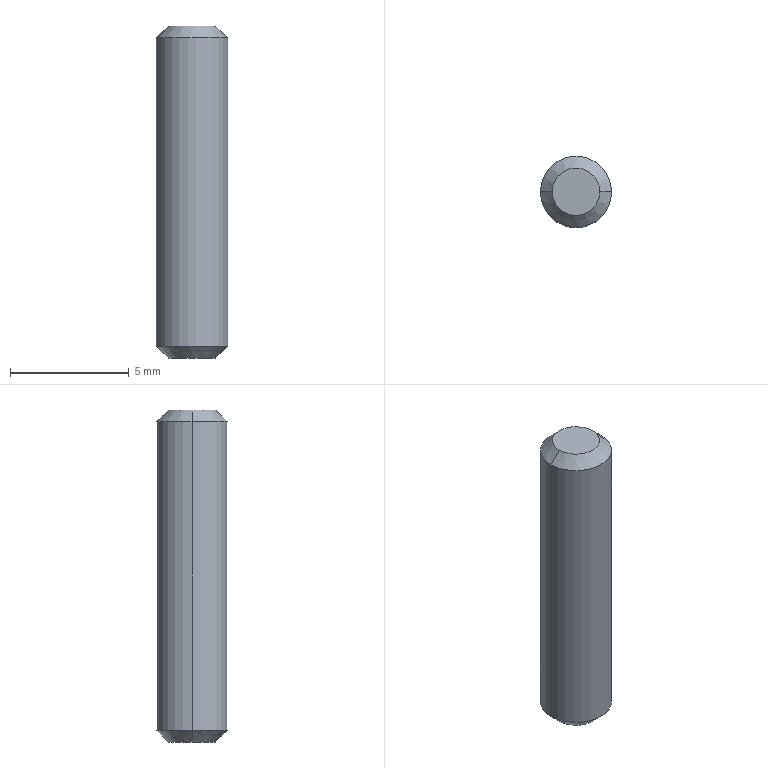Part | SolidWorks | features Chamfer 1, Extrusion 1 | 1 solid | 8 faces | box 3 x 3 x 14 mm | volume 96.866 mm3 | cone 4 | cylinder 2 | plane 2 | commonest cylinder face diameters 3 x2
STEP:
#1=CARTESIAN_POINT('',(1.,0.,14.));
#2=VERTEX_POINT('',#1);
#3=CARTESIAN_POINT('',(-1.,0.,14.));
#4=VERTEX_POINT('',#3);
#5=CARTESIAN_POINT('',(0.,0.,14.));
#6=DIRECTION('',(0.,0.,1.));
#7=DIRECTION('',(1.,0.,0.));
#8=AXIS2_PLACEMENT_3D('',#5,#6,#7);
#9=CIRCLE('',#8,1.);
#10=EDGE_CURVE('',#2,#4,#9,.T.);
#11=ORIENTED_EDGE('',*,*,#10,.F.);
#12=CARTESIAN_POINT('',(1.5,0.,13.5));
#13=VERTEX_POINT('',#12);
#14=CARTESIAN_POINT('',(1.,0.,14.));
#15=DIRECTION('',(0.7071,0.,-0.7071));
#16=VECTOR('',#15,1000.);
#17=LINE('',#14,#16);
#18=EDGE_CURVE('',#2,#13,#17,.T.);
#19=ORIENTED_EDGE('',*,*,#18,.T.);
#20=CARTESIAN_POINT('',(-1.5,0.,13.5));
#21=VERTEX_POINT('',#20);
#22=CARTESIAN_POINT('',(0.,0.,13.5));
#23=DIRECTION('',(0.,0.,-1.));
#24=DIRECTION('',(1.,0.,0.));
#25=AXIS2_PLACEMENT_3D('',#22,#23,#24);
#26=CIRCLE('',#25,1.5);
#27=EDGE_CURVE('',#21,#13,#26,.T.);
#28=ORIENTED_EDGE('',*,*,#27,.F.);
#29=CARTESIAN_POINT('',(-1.,0.,14.));
#30=DIRECTION('',(-0.7071,0.,-0.7071));
#31=VECTOR('',#30,1000.);
#32=LINE('',#29,#31);
#33=EDGE_CURVE('',#4,#21,#32,.T.);
#34=ORIENTED_EDGE('',*,*,#33,.F.);
#35=EDGE_LOOP('',(#11,#19,#28,#34));
#36=FACE_OUTER_BOUND('',#35,.T.);
#37=CARTESIAN_POINT('',(0.,0.,14.));
#38=DIRECTION('',(0.,0.,-1.));
#39=DIRECTION('',(-1.,0.,0.));
#40=AXIS2_PLACEMENT_3D('',#37,#38,#39);
#41=CONICAL_SURFACE('',#40,1.,0.7854);
#42=ADVANCED_FACE('',(#36),#41,.T.);
#43=CARTESIAN_POINT('',(-1.,0.,0.));
#44=VERTEX_POINT('',#43);
#45=CARTESIAN_POINT('',(1.,0.,0.));
#46=VERTEX_POINT('',#45);
#47=CARTESIAN_POINT('',(0.,0.,0.));
#48=DIRECTION('',(0.,0.,-1.));
#49=DIRECTION('',(1.,0.,0.));
#50=AXIS2_PLACEMENT_3D('',#47,#48,#49);
#51=CIRCLE('',#50,1.);
#52=EDGE_CURVE('',#44,#46,#51,.T.);
#53=ORIENTED_EDGE('',*,*,#52,.F.);
#54=CARTESIAN_POINT('',(-1.5,0.,0.5));
#55=VERTEX_POINT('',#54);
#56=CARTESIAN_POINT('',(-1.5,0.,0.5));
#57=DIRECTION('',(-0.7071,0.,0.7071));
#58=VECTOR('',#57,1000.);
#59=LINE('',#56,#58);
#60=EDGE_CURVE('',#44,#55,#59,.T.);
#61=ORIENTED_EDGE('',*,*,#60,.T.);
#62=CARTESIAN_POINT('',(1.5,0.,0.5));
#63=VERTEX_POINT('',#62);
#64=CARTESIAN_POINT('',(0.,0.,0.5));
#65=DIRECTION('',(0.,0.,1.));
#66=DIRECTION('',(1.,0.,0.));
#67=AXIS2_PLACEMENT_3D('',#64,#65,#66);
#68=CIRCLE('',#67,1.5);
#69=EDGE_CURVE('',#63,#55,#68,.T.);
#70=ORIENTED_EDGE('',*,*,#69,.F.);
#71=CARTESIAN_POINT('',(1.5,0.,0.5));
#72=DIRECTION('',(0.7071,0.,0.7071));
#73=VECTOR('',#72,1000.);
#74=LINE('',#71,#73);
#75=EDGE_CURVE('',#46,#63,#74,.T.);
#76=ORIENTED_EDGE('',*,*,#75,.F.);
#77=EDGE_LOOP('',(#53,#61,#70,#76));
#78=FACE_OUTER_BOUND('',#77,.T.);
#79=CARTESIAN_POINT('',(0.,0.,0.5));
#80=DIRECTION('',(0.,0.,1.));
#81=DIRECTION('',(1.,0.,0.));
#82=AXIS2_PLACEMENT_3D('',#79,#80,#81);
#83=CONICAL_SURFACE('',#82,1.5,0.7854);
#84=ADVANCED_FACE('',(#78),#83,.T.);
#85=ORIENTED_EDGE('',*,*,#27,.T.);
#86=CARTESIAN_POINT('',(1.5,0.,14.));
#87=DIRECTION('',(0.,0.,-1.));
#88=VECTOR('',#87,1000.);
#89=LINE('',#86,#88);
#90=EDGE_CURVE('',#13,#63,#89,.T.);
#91=ORIENTED_EDGE('',*,*,#90,.T.);
#92=ORIENTED_EDGE('',*,*,#69,.T.);
#93=CARTESIAN_POINT('',(-1.5,0.,14.));
#94=DIRECTION('',(0.,0.,-1.));
#95=VECTOR('',#94,1000.);
#96=LINE('',#93,#95);
#97=EDGE_CURVE('',#21,#55,#96,.T.);
#98=ORIENTED_EDGE('',*,*,#97,.F.);
#99=EDGE_LOOP('',(#85,#91,#92,#98));
#100=FACE_OUTER_BOUND('',#99,.T.);
#101=CARTESIAN_POINT('',(0.,0.,14.));
#102=DIRECTION('',(0.,0.,-1.));
#103=DIRECTION('',(-1.,0.,0.));
#104=AXIS2_PLACEMENT_3D('',#101,#102,#103);
#105=CYLINDRICAL_SURFACE('',#104,1.5);
#106=ADVANCED_FACE('',(#100),#105,.T.);
#107=ORIENTED_EDGE('',*,*,#90,.F.);
#108=CARTESIAN_POINT('',(0.,0.,13.5));
#109=DIRECTION('',(0.,0.,-1.));
#110=DIRECTION('',(1.,0.,0.));
#111=AXIS2_PLACEMENT_3D('',#108,#109,#110);
#112=CIRCLE('',#111,1.5);
#113=EDGE_CURVE('',#13,#21,#112,.T.);
#114=ORIENTED_EDGE('',*,*,#113,.T.);
#115=ORIENTED_EDGE('',*,*,#97,.T.);
#116=CARTESIAN_POINT('',(0.,0.,0.5));
#117=DIRECTION('',(0.,0.,1.));
#118=DIRECTION('',(1.,0.,0.));
#119=AXIS2_PLACEMENT_3D('',#116,#117,#118);
#120=CIRCLE('',#119,1.5);
#121=EDGE_CURVE('',#55,#63,#120,.T.);
#122=ORIENTED_EDGE('',*,*,#121,.T.);
#123=EDGE_LOOP('',(#107,#114,#115,#122));
#124=FACE_OUTER_BOUND('',#123,.T.);
#125=CARTESIAN_POINT('',(0.,0.,14.));
#126=DIRECTION('',(0.,0.,-1.));
#127=DIRECTION('',(-1.,0.,0.));
#128=AXIS2_PLACEMENT_3D('',#125,#126,#127);
#129=CYLINDRICAL_SURFACE('',#128,1.5);
#130=ADVANCED_FACE('',(#124),#129,.T.);
#131=CARTESIAN_POINT('',(0.,0.,14.));
#132=DIRECTION('',(0.,0.,1.));
#133=DIRECTION('',(1.,0.,0.));
#134=AXIS2_PLACEMENT_3D('',#131,#132,#133);
#135=CIRCLE('',#134,1.);
#136=EDGE_CURVE('',#4,#2,#135,.T.);
#137=ORIENTED_EDGE('',*,*,#136,.T.);
#138=ORIENTED_EDGE('',*,*,#10,.T.);
#139=EDGE_LOOP('',(#137,#138));
#140=FACE_OUTER_BOUND('',#139,.T.);
#141=CARTESIAN_POINT('',(0.,0.,14.));
#142=DIRECTION('',(0.,0.,1.));
#143=DIRECTION('',(1.,0.,0.));
#144=AXIS2_PLACEMENT_3D('',#141,#142,#143);
#145=PLANE('',#144);
#146=ADVANCED_FACE('',(#140),#145,.T.);
#147=CARTESIAN_POINT('',(0.,0.,0.));
#148=DIRECTION('',(0.,0.,-1.));
#149=DIRECTION('',(1.,0.,0.));
#150=AXIS2_PLACEMENT_3D('',#147,#148,#149);
#151=CIRCLE('',#150,1.);
#152=EDGE_CURVE('',#46,#44,#151,.T.);
#153=ORIENTED_EDGE('',*,*,#152,.T.);
#154=ORIENTED_EDGE('',*,*,#52,.T.);
#155=EDGE_LOOP('',(#153,#154));
#156=FACE_OUTER_BOUND('',#155,.T.);
#157=CARTESIAN_POINT('',(0.,0.,0.));
#158=DIRECTION('',(0.,0.,1.));
#159=DIRECTION('',(1.,0.,0.));
#160=AXIS2_PLACEMENT_3D('',#157,#158,#159);
#161=PLANE('',#160);
#162=ADVANCED_FACE('',(#156),#161,.F.);
#163=ORIENTED_EDGE('',*,*,#60,.F.);
#164=ORIENTED_EDGE('',*,*,#152,.F.);
#165=ORIENTED_EDGE('',*,*,#75,.T.);
#166=ORIENTED_EDGE('',*,*,#121,.F.);
#167=EDGE_LOOP('',(#163,#164,#165,#166));
#168=FACE_OUTER_BOUND('',#167,.T.);
#169=CARTESIAN_POINT('',(0.,0.,0.5));
#170=DIRECTION('',(0.,0.,1.));
#171=DIRECTION('',(1.,0.,0.));
#172=AXIS2_PLACEMENT_3D('',#169,#170,#171);
#173=CONICAL_SURFACE('',#172,1.5,0.7854);
#174=ADVANCED_FACE('',(#168),#173,.T.);
#175=ORIENTED_EDGE('',*,*,#18,.F.);
#176=ORIENTED_EDGE('',*,*,#136,.F.);
#177=ORIENTED_EDGE('',*,*,#33,.T.);
#178=ORIENTED_EDGE('',*,*,#113,.F.);
#179=EDGE_LOOP('',(#175,#176,#177,#178));
#180=FACE_OUTER_BOUND('',#179,.T.);
#181=CARTESIAN_POINT('',(0.,0.,14.));
#182=DIRECTION('',(0.,0.,-1.));
#183=DIRECTION('',(-1.,0.,0.));
#184=AXIS2_PLACEMENT_3D('',#181,#182,#183);
#185=CONICAL_SURFACE('',#184,1.,0.7854);
#186=ADVANCED_FACE('',(#180),#185,.T.);
#187=CLOSED_SHELL('',(#42,#84,#106,#130,#146,#162,#174,#186));
#188=MANIFOLD_SOLID_BREP('',#187);
#189=CARTESIAN_POINT('',(0.,0.,0.));
#190=DIRECTION('',(0.,0.,1.));
#191=DIRECTION('',(1.,0.,0.));
#192=AXIS2_PLACEMENT_3D('',#189,#190,#191);
#193=(LENGTH_UNIT()NAMED_UNIT(*)SI_UNIT(.MILLI.,.METRE.));
#194=UNCERTAINTY_MEASURE_WITH_UNIT(LENGTH_MEASURE(0.00001),#193,'','');
#195=(NAMED_UNIT(*)PLANE_ANGLE_UNIT()SI_UNIT($,.RADIAN.));
#196=(NAMED_UNIT(*)SI_UNIT($,.STERADIAN.)SOLID_ANGLE_UNIT());
#197=(GEOMETRIC_REPRESENTATION_CONTEXT(3)GLOBAL_UNCERTAINTY_ASSIGNED_CONTEXT((#194))GLOBAL_UNIT_ASSIGNED_CONTEXT((#193,#195,#196))REPRESENTATION_CONTEXT('',''));
#198=ADVANCED_BREP_SHAPE_REPRESENTATION('',(#188,#192),#197);